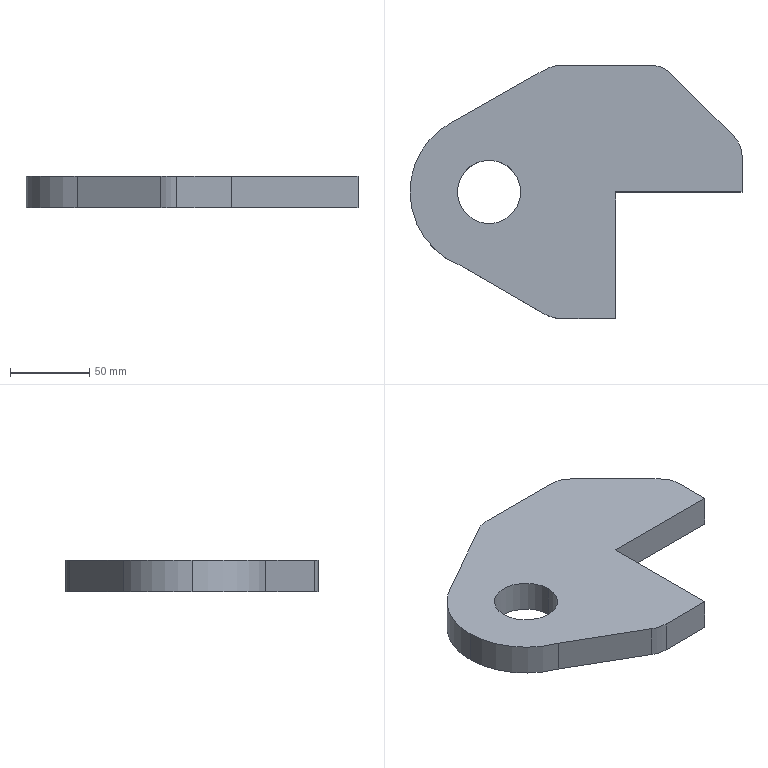Part | SolidWorks | features BaseBody 1 | 1 solid | 18 faces | box 210 x 160 x 20 mm | volume 396110 mm3 | plane 10 | cylinder 8 | commonest cylinder face diameters 40 x4 34.445 x2 100 x2
STEP:
#1=CARTESIAN_POINT('',(-20.,0.,10.));
#2=VERTEX_POINT('',#1);
#3=CARTESIAN_POINT('',(20.,0.,10.));
#4=VERTEX_POINT('',#3);
#5=CARTESIAN_POINT('',(0.,0.,10.));
#6=DIRECTION('',(0.,0.,1.));
#7=DIRECTION('',(1.,0.,0.));
#8=AXIS2_PLACEMENT_3D('',#5,#6,#7);
#9=CIRCLE('',#8,20.);
#10=EDGE_CURVE('',#2,#4,#9,.T.);
#11=ORIENTED_EDGE('',*,*,#10,.T.);
#12=CARTESIAN_POINT('',(20.,0.,-10.));
#13=VERTEX_POINT('',#12);
#14=CARTESIAN_POINT('',(20.,0.,10.));
#15=DIRECTION('',(0.,0.,-1.));
#16=VECTOR('',#15,1000.);
#17=LINE('',#14,#16);
#18=EDGE_CURVE('',#4,#13,#17,.T.);
#19=ORIENTED_EDGE('',*,*,#18,.T.);
#20=CARTESIAN_POINT('',(-20.,0.,-10.));
#21=VERTEX_POINT('',#20);
#22=CARTESIAN_POINT('',(0.,0.,-10.));
#23=DIRECTION('',(0.,0.,1.));
#24=DIRECTION('',(1.,0.,0.));
#25=AXIS2_PLACEMENT_3D('',#22,#23,#24);
#26=CIRCLE('',#25,20.);
#27=EDGE_CURVE('',#21,#13,#26,.T.);
#28=ORIENTED_EDGE('',*,*,#27,.F.);
#29=CARTESIAN_POINT('',(-20.,0.,10.));
#30=DIRECTION('',(0.,0.,-1.));
#31=VECTOR('',#30,1000.);
#32=LINE('',#29,#31);
#33=EDGE_CURVE('',#2,#21,#32,.T.);
#34=ORIENTED_EDGE('',*,*,#33,.F.);
#35=EDGE_LOOP('',(#11,#19,#28,#34));
#36=FACE_OUTER_BOUND('',#35,.T.);
#37=CARTESIAN_POINT('',(0.,0.,10.));
#38=DIRECTION('',(0.,0.,-1.));
#39=DIRECTION('',(-1.,0.,0.));
#40=AXIS2_PLACEMENT_3D('',#37,#38,#39);
#41=CYLINDRICAL_SURFACE('',#40,20.);
#42=ADVANCED_FACE('',(#36),#41,.F.);
#43=CARTESIAN_POINT('',(-50.,0.,10.));
#44=VERTEX_POINT('',#43);
#45=CARTESIAN_POINT('',(-17.72,-46.755,10.));
#46=VERTEX_POINT('',#45);
#47=CARTESIAN_POINT('',(0.,0.,10.));
#48=DIRECTION('',(0.,0.,1.));
#49=DIRECTION('',(1.,0.,0.));
#50=AXIS2_PLACEMENT_3D('',#47,#48,#49);
#51=CIRCLE('',#50,50.);
#52=EDGE_CURVE('',#44,#46,#51,.T.);
#53=ORIENTED_EDGE('',*,*,#52,.F.);
#54=CARTESIAN_POINT('',(-50.,0.,-10.));
#55=VERTEX_POINT('',#54);
#56=CARTESIAN_POINT('',(-50.,0.,10.));
#57=DIRECTION('',(0.,0.,-1.));
#58=VECTOR('',#57,1000.);
#59=LINE('',#56,#58);
#60=EDGE_CURVE('',#44,#55,#59,.T.);
#61=ORIENTED_EDGE('',*,*,#60,.T.);
#62=CARTESIAN_POINT('',(-17.72,-46.755,-10.));
#63=VERTEX_POINT('',#62);
#64=CARTESIAN_POINT('',(0.,0.,-10.));
#65=DIRECTION('',(0.,0.,1.));
#66=DIRECTION('',(1.,0.,0.));
#67=AXIS2_PLACEMENT_3D('',#64,#65,#66);
#68=CIRCLE('',#67,50.);
#69=EDGE_CURVE('',#55,#63,#68,.T.);
#70=ORIENTED_EDGE('',*,*,#69,.T.);
#71=CARTESIAN_POINT('',(-17.72,-46.755,10.));
#72=DIRECTION('',(0.,0.,-1.));
#73=VECTOR('',#72,1000.);
#74=LINE('',#71,#73);
#75=EDGE_CURVE('',#46,#63,#74,.T.);
#76=ORIENTED_EDGE('',*,*,#75,.F.);
#77=EDGE_LOOP('',(#53,#61,#70,#76));
#78=FACE_OUTER_BOUND('',#77,.T.);
#79=CARTESIAN_POINT('',(0.,0.,10.));
#80=DIRECTION('',(0.,0.,-1.));
#81=DIRECTION('',(-1.,0.,0.));
#82=AXIS2_PLACEMENT_3D('',#79,#80,#81);
#83=CYLINDRICAL_SURFACE('',#82,50.);
#84=ADVANCED_FACE('',(#78),#83,.T.);
#85=CARTESIAN_POINT('',(80.,0.,10.));
#86=VERTEX_POINT('',#85);
#87=CARTESIAN_POINT('',(80.,0.,-10.));
#88=VERTEX_POINT('',#87);
#89=CARTESIAN_POINT('',(80.,0.,10.));
#90=DIRECTION('',(0.,0.,-1.));
#91=VECTOR('',#90,1000.);
#92=LINE('',#89,#91);
#93=EDGE_CURVE('',#86,#88,#92,.T.);
#94=ORIENTED_EDGE('',*,*,#93,.F.);
#95=CARTESIAN_POINT('',(80.,-80.,10.));
#96=VERTEX_POINT('',#95);
#97=CARTESIAN_POINT('',(80.,80.,10.));
#98=DIRECTION('',(0.,1.,0.));
#99=VECTOR('',#98,1000.);
#100=LINE('',#97,#99);
#101=EDGE_CURVE('',#96,#86,#100,.T.);
#102=ORIENTED_EDGE('',*,*,#101,.F.);
#103=CARTESIAN_POINT('',(80.,-80.,-10.));
#104=VERTEX_POINT('',#103);
#105=CARTESIAN_POINT('',(80.,-80.,10.));
#106=DIRECTION('',(0.,0.,-1.));
#107=VECTOR('',#106,1000.);
#108=LINE('',#105,#107);
#109=EDGE_CURVE('',#96,#104,#108,.T.);
#110=ORIENTED_EDGE('',*,*,#109,.T.);
#111=CARTESIAN_POINT('',(80.,80.,-10.));
#112=DIRECTION('',(0.,1.,0.));
#113=VECTOR('',#112,1000.);
#114=LINE('',#111,#113);
#115=EDGE_CURVE('',#104,#88,#114,.T.);
#116=ORIENTED_EDGE('',*,*,#115,.T.);
#117=EDGE_LOOP('',(#94,#102,#110,#116));
#118=FACE_OUTER_BOUND('',#117,.T.);
#119=CARTESIAN_POINT('',(80.,80.,10.));
#120=DIRECTION('',(-1.,0.,0.));
#121=DIRECTION('',(0.,-1.,0.));
#122=AXIS2_PLACEMENT_3D('',#119,#120,#121);
#123=PLANE('',#122);
#124=ADVANCED_FACE('',(#118),#123,.F.);
#125=CARTESIAN_POINT('',(45.256,80.,10.));
#126=VERTEX_POINT('',#125);
#127=CARTESIAN_POINT('',(35.423,77.416,10.));
#128=VERTEX_POINT('',#127);
#129=CARTESIAN_POINT('',(45.256,60.,10.));
#130=DIRECTION('',(0.,0.,1.));
#131=DIRECTION('',(1.,0.,0.));
#132=AXIS2_PLACEMENT_3D('',#129,#130,#131);
#133=CIRCLE('',#132,20.);
#134=EDGE_CURVE('',#126,#128,#133,.T.);
#135=ORIENTED_EDGE('',*,*,#134,.T.);
#136=CARTESIAN_POINT('',(-24.581,43.54,10.));
#137=VERTEX_POINT('',#136);
#138=CARTESIAN_POINT('',(35.423,77.416,10.));
#139=DIRECTION('',(-0.8708,-0.4916,0.));
#140=VECTOR('',#139,1000.);
#141=LINE('',#138,#140);
#142=EDGE_CURVE('',#128,#137,#141,.T.);
#143=ORIENTED_EDGE('',*,*,#142,.T.);
#144=CARTESIAN_POINT('',(0.,0.,10.));
#145=DIRECTION('',(0.,0.,1.));
#146=DIRECTION('',(1.,0.,0.));
#147=AXIS2_PLACEMENT_3D('',#144,#145,#146);
#148=CIRCLE('',#147,50.);
#149=EDGE_CURVE('',#137,#44,#148,.T.);
#150=ORIENTED_EDGE('',*,*,#149,.T.);
#151=ORIENTED_EDGE('',*,*,#52,.T.);
#152=CARTESIAN_POINT('',(35.366,-77.331,10.));
#153=VERTEX_POINT('',#152);
#154=CARTESIAN_POINT('',(35.366,-77.331,10.));
#155=DIRECTION('',(0.8665,-0.4991,0.));
#156=VECTOR('',#155,1000.);
#157=LINE('',#154,#156);
#158=EDGE_CURVE('',#46,#153,#157,.T.);
#159=ORIENTED_EDGE('',*,*,#158,.T.);
#160=CARTESIAN_POINT('',(45.348,-80.,10.));
#161=VERTEX_POINT('',#160);
#162=CARTESIAN_POINT('',(45.348,-60.,10.));
#163=DIRECTION('',(0.,0.,1.));
#164=DIRECTION('',(1.,0.,0.));
#165=AXIS2_PLACEMENT_3D('',#162,#163,#164);
#166=CIRCLE('',#165,20.);
#167=EDGE_CURVE('',#153,#161,#166,.T.);
#168=ORIENTED_EDGE('',*,*,#167,.T.);
#169=CARTESIAN_POINT('',(80.,-80.,10.));
#170=DIRECTION('',(1.,0.,0.));
#171=VECTOR('',#170,1000.);
#172=LINE('',#169,#171);
#173=EDGE_CURVE('',#161,#96,#172,.T.);
#174=ORIENTED_EDGE('',*,*,#173,.T.);
#175=ORIENTED_EDGE('',*,*,#101,.T.);
#176=CARTESIAN_POINT('',(160.,0.,10.));
#177=VERTEX_POINT('',#176);
#178=CARTESIAN_POINT('',(160.,0.,10.));
#179=DIRECTION('',(1.,0.,0.));
#180=VECTOR('',#179,1000.);
#181=LINE('',#178,#180);
#182=EDGE_CURVE('',#86,#177,#181,.T.);
#183=ORIENTED_EDGE('',*,*,#182,.T.);
#184=CARTESIAN_POINT('',(160.,22.866,10.));
#185=VERTEX_POINT('',#184);
#186=CARTESIAN_POINT('',(160.,22.866,10.));
#187=DIRECTION('',(0.,1.,0.));
#188=VECTOR('',#187,1000.);
#189=LINE('',#186,#188);
#190=EDGE_CURVE('',#177,#185,#189,.T.);
#191=ORIENTED_EDGE('',*,*,#190,.T.);
#192=CARTESIAN_POINT('',(154.956,35.044,10.));
#193=VERTEX_POINT('',#192);
#194=CARTESIAN_POINT('',(142.778,22.866,10.));
#195=DIRECTION('',(0.,0.,1.));
#196=DIRECTION('',(-1.,0.,0.));
#197=AXIS2_PLACEMENT_3D('',#194,#195,#196);
#198=CIRCLE('',#197,17.222);
#199=EDGE_CURVE('',#185,#193,#198,.T.);
#200=ORIENTED_EDGE('',*,*,#199,.T.);
#201=CARTESIAN_POINT('',(115.044,74.956,10.));
#202=VERTEX_POINT('',#201);
#203=CARTESIAN_POINT('',(115.044,74.956,10.));
#204=DIRECTION('',(-0.7071,0.7071,0.));
#205=VECTOR('',#204,1000.);
#206=LINE('',#203,#205);
#207=EDGE_CURVE('',#193,#202,#206,.T.);
#208=ORIENTED_EDGE('',*,*,#207,.T.);
#209=CARTESIAN_POINT('',(102.866,80.,10.));
#210=VERTEX_POINT('',#209);
#211=CARTESIAN_POINT('',(102.866,62.778,10.));
#212=DIRECTION('',(0.,0.,1.));
#213=DIRECTION('',(-1.,0.,0.));
#214=AXIS2_PLACEMENT_3D('',#211,#212,#213);
#215=CIRCLE('',#214,17.222);
#216=EDGE_CURVE('',#202,#210,#215,.T.);
#217=ORIENTED_EDGE('',*,*,#216,.T.);
#218=CARTESIAN_POINT('',(80.,80.,10.));
#219=DIRECTION('',(-1.,0.,0.));
#220=VECTOR('',#219,1000.);
#221=LINE('',#218,#220);
#222=EDGE_CURVE('',#210,#126,#221,.T.);
#223=ORIENTED_EDGE('',*,*,#222,.T.);
#224=EDGE_LOOP('',(#135,#143,#150,#151,#159,#168,#174,#175,#183,#191,#200,#208,#217,#223));
#225=FACE_OUTER_BOUND('',#224,.T.);
#226=ORIENTED_EDGE('',*,*,#10,.F.);
#227=CARTESIAN_POINT('',(0.,0.,10.));
#228=DIRECTION('',(0.,0.,1.));
#229=DIRECTION('',(1.,0.,0.));
#230=AXIS2_PLACEMENT_3D('',#227,#228,#229);
#231=CIRCLE('',#230,20.);
#232=EDGE_CURVE('',#4,#2,#231,.T.);
#233=ORIENTED_EDGE('',*,*,#232,.F.);
#234=EDGE_LOOP('',(#226,#233));
#235=FACE_BOUND('',#234,.T.);
#236=CARTESIAN_POINT('',(45.256,60.,10.));
#237=DIRECTION('',(0.,0.,1.));
#238=DIRECTION('',(1.,0.,0.));
#239=AXIS2_PLACEMENT_3D('',#236,#237,#238);
#240=PLANE('',#239);
#241=ADVANCED_FACE('',(#225,#235),#240,.T.);
#242=CARTESIAN_POINT('',(45.256,80.,-10.));
#243=VERTEX_POINT('',#242);
#244=CARTESIAN_POINT('',(35.423,77.416,-10.));
#245=VERTEX_POINT('',#244);
#246=CARTESIAN_POINT('',(45.256,60.,-10.));
#247=DIRECTION('',(0.,0.,1.));
#248=DIRECTION('',(1.,0.,0.));
#249=AXIS2_PLACEMENT_3D('',#246,#247,#248);
#250=CIRCLE('',#249,20.);
#251=EDGE_CURVE('',#243,#245,#250,.T.);
#252=ORIENTED_EDGE('',*,*,#251,.F.);
#253=CARTESIAN_POINT('',(102.866,80.,-10.));
#254=VERTEX_POINT('',#253);
#255=CARTESIAN_POINT('',(80.,80.,-10.));
#256=DIRECTION('',(-1.,0.,0.));
#257=VECTOR('',#256,1000.);
#258=LINE('',#255,#257);
#259=EDGE_CURVE('',#254,#243,#258,.T.);
#260=ORIENTED_EDGE('',*,*,#259,.F.);
#261=CARTESIAN_POINT('',(115.044,74.956,-10.));
#262=VERTEX_POINT('',#261);
#263=CARTESIAN_POINT('',(102.866,62.778,-10.));
#264=DIRECTION('',(0.,0.,1.));
#265=DIRECTION('',(-1.,0.,0.));
#266=AXIS2_PLACEMENT_3D('',#263,#264,#265);
#267=CIRCLE('',#266,17.222);
#268=EDGE_CURVE('',#262,#254,#267,.T.);
#269=ORIENTED_EDGE('',*,*,#268,.F.);
#270=CARTESIAN_POINT('',(154.956,35.044,-10.));
#271=VERTEX_POINT('',#270);
#272=CARTESIAN_POINT('',(115.044,74.956,-10.));
#273=DIRECTION('',(-0.7071,0.7071,0.));
#274=VECTOR('',#273,1000.);
#275=LINE('',#272,#274);
#276=EDGE_CURVE('',#271,#262,#275,.T.);
#277=ORIENTED_EDGE('',*,*,#276,.F.);
#278=CARTESIAN_POINT('',(160.,22.866,-10.));
#279=VERTEX_POINT('',#278);
#280=CARTESIAN_POINT('',(142.778,22.866,-10.));
#281=DIRECTION('',(0.,0.,1.));
#282=DIRECTION('',(-1.,0.,0.));
#283=AXIS2_PLACEMENT_3D('',#280,#281,#282);
#284=CIRCLE('',#283,17.222);
#285=EDGE_CURVE('',#279,#271,#284,.T.);
#286=ORIENTED_EDGE('',*,*,#285,.F.);
#287=CARTESIAN_POINT('',(160.,0.,-10.));
#288=VERTEX_POINT('',#287);
#289=CARTESIAN_POINT('',(160.,22.866,-10.));
#290=DIRECTION('',(0.,1.,0.));
#291=VECTOR('',#290,1000.);
#292=LINE('',#289,#291);
#293=EDGE_CURVE('',#288,#279,#292,.T.);
#294=ORIENTED_EDGE('',*,*,#293,.F.);
#295=CARTESIAN_POINT('',(160.,0.,-10.));
#296=DIRECTION('',(1.,0.,0.));
#297=VECTOR('',#296,1000.);
#298=LINE('',#295,#297);
#299=EDGE_CURVE('',#88,#288,#298,.T.);
#300=ORIENTED_EDGE('',*,*,#299,.F.);
#301=ORIENTED_EDGE('',*,*,#115,.F.);
#302=CARTESIAN_POINT('',(45.348,-80.,-10.));
#303=VERTEX_POINT('',#302);
#304=CARTESIAN_POINT('',(80.,-80.,-10.));
#305=DIRECTION('',(1.,0.,0.));
#306=VECTOR('',#305,1000.);
#307=LINE('',#304,#306);
#308=EDGE_CURVE('',#303,#104,#307,.T.);
#309=ORIENTED_EDGE('',*,*,#308,.F.);
#310=CARTESIAN_POINT('',(35.366,-77.331,-10.));
#311=VERTEX_POINT('',#310);
#312=CARTESIAN_POINT('',(45.348,-60.,-10.));
#313=DIRECTION('',(0.,0.,1.));
#314=DIRECTION('',(1.,0.,0.));
#315=AXIS2_PLACEMENT_3D('',#312,#313,#314);
#316=CIRCLE('',#315,20.);
#317=EDGE_CURVE('',#311,#303,#316,.T.);
#318=ORIENTED_EDGE('',*,*,#317,.F.);
#319=CARTESIAN_POINT('',(35.366,-77.331,-10.));
#320=DIRECTION('',(0.8665,-0.4991,0.));
#321=VECTOR('',#320,1000.);
#322=LINE('',#319,#321);
#323=EDGE_CURVE('',#63,#311,#322,.T.);
#324=ORIENTED_EDGE('',*,*,#323,.F.);
#325=ORIENTED_EDGE('',*,*,#69,.F.);
#326=CARTESIAN_POINT('',(-24.581,43.54,-10.));
#327=VERTEX_POINT('',#326);
#328=CARTESIAN_POINT('',(0.,0.,-10.));
#329=DIRECTION('',(0.,0.,1.));
#330=DIRECTION('',(1.,0.,0.));
#331=AXIS2_PLACEMENT_3D('',#328,#329,#330);
#332=CIRCLE('',#331,50.);
#333=EDGE_CURVE('',#327,#55,#332,.T.);
#334=ORIENTED_EDGE('',*,*,#333,.F.);
#335=CARTESIAN_POINT('',(35.423,77.416,-10.));
#336=DIRECTION('',(-0.8708,-0.4916,0.));
#337=VECTOR('',#336,1000.);
#338=LINE('',#335,#337);
#339=EDGE_CURVE('',#245,#327,#338,.T.);
#340=ORIENTED_EDGE('',*,*,#339,.F.);
#341=EDGE_LOOP('',(#252,#260,#269,#277,#286,#294,#300,#301,#309,#318,#324,#325,#334,#340));
#342=FACE_OUTER_BOUND('',#341,.T.);
#343=ORIENTED_EDGE('',*,*,#27,.T.);
#344=CARTESIAN_POINT('',(0.,0.,-10.));
#345=DIRECTION('',(0.,0.,1.));
#346=DIRECTION('',(1.,0.,0.));
#347=AXIS2_PLACEMENT_3D('',#344,#345,#346);
#348=CIRCLE('',#347,20.);
#349=EDGE_CURVE('',#13,#21,#348,.T.);
#350=ORIENTED_EDGE('',*,*,#349,.T.);
#351=EDGE_LOOP('',(#343,#350));
#352=FACE_BOUND('',#351,.T.);
#353=CARTESIAN_POINT('',(45.256,60.,-10.));
#354=DIRECTION('',(0.,0.,1.));
#355=DIRECTION('',(1.,0.,0.));
#356=AXIS2_PLACEMENT_3D('',#353,#354,#355);
#357=PLANE('',#356);
#358=ADVANCED_FACE('',(#342,#352),#357,.F.);
#359=ORIENTED_EDGE('',*,*,#251,.T.);
#360=CARTESIAN_POINT('',(35.423,77.416,10.));
#361=DIRECTION('',(0.,0.,-1.));
#362=VECTOR('',#361,1000.);
#363=LINE('',#360,#362);
#364=EDGE_CURVE('',#128,#245,#363,.T.);
#365=ORIENTED_EDGE('',*,*,#364,.F.);
#366=ORIENTED_EDGE('',*,*,#134,.F.);
#367=CARTESIAN_POINT('',(45.256,80.,10.));
#368=DIRECTION('',(0.,0.,-1.));
#369=VECTOR('',#368,1000.);
#370=LINE('',#367,#369);
#371=EDGE_CURVE('',#126,#243,#370,.T.);
#372=ORIENTED_EDGE('',*,*,#371,.T.);
#373=EDGE_LOOP('',(#359,#365,#366,#372));
#374=FACE_OUTER_BOUND('',#373,.T.);
#375=CARTESIAN_POINT('',(45.256,60.,10.));
#376=DIRECTION('',(0.,0.,-1.));
#377=DIRECTION('',(-1.,0.,0.));
#378=AXIS2_PLACEMENT_3D('',#375,#376,#377);
#379=CYLINDRICAL_SURFACE('',#378,20.);
#380=ADVANCED_FACE('',(#374),#379,.T.);
#381=ORIENTED_EDGE('',*,*,#339,.T.);
#382=CARTESIAN_POINT('',(-24.581,43.54,10.));
#383=DIRECTION('',(0.,0.,-1.));
#384=VECTOR('',#383,1000.);
#385=LINE('',#382,#384);
#386=EDGE_CURVE('',#137,#327,#385,.T.);
#387=ORIENTED_EDGE('',*,*,#386,.F.);
#388=ORIENTED_EDGE('',*,*,#142,.F.);
#389=ORIENTED_EDGE('',*,*,#364,.T.);
#390=EDGE_LOOP('',(#381,#387,#388,#389));
#391=FACE_OUTER_BOUND('',#390,.T.);
#392=CARTESIAN_POINT('',(35.423,77.416,10.));
#393=DIRECTION('',(0.4916,-0.8708,0.));
#394=DIRECTION('',(0.8708,0.4916,0.));
#395=AXIS2_PLACEMENT_3D('',#392,#393,#394);
#396=PLANE('',#395);
#397=ADVANCED_FACE('',(#391),#396,.F.);
#398=ORIENTED_EDGE('',*,*,#60,.F.);
#399=ORIENTED_EDGE('',*,*,#149,.F.);
#400=ORIENTED_EDGE('',*,*,#386,.T.);
#401=ORIENTED_EDGE('',*,*,#333,.T.);
#402=EDGE_LOOP('',(#398,#399,#400,#401));
#403=FACE_OUTER_BOUND('',#402,.T.);
#404=CARTESIAN_POINT('',(0.,0.,10.));
#405=DIRECTION('',(0.,0.,-1.));
#406=DIRECTION('',(-1.,0.,0.));
#407=AXIS2_PLACEMENT_3D('',#404,#405,#406);
#408=CYLINDRICAL_SURFACE('',#407,50.);
#409=ADVANCED_FACE('',(#403),#408,.T.);
#410=ORIENTED_EDGE('',*,*,#323,.T.);
#411=CARTESIAN_POINT('',(35.366,-77.331,10.));
#412=DIRECTION('',(0.,0.,-1.));
#413=VECTOR('',#412,1000.);
#414=LINE('',#411,#413);
#415=EDGE_CURVE('',#153,#311,#414,.T.);
#416=ORIENTED_EDGE('',*,*,#415,.F.);
#417=ORIENTED_EDGE('',*,*,#158,.F.);
#418=ORIENTED_EDGE('',*,*,#75,.T.);
#419=EDGE_LOOP('',(#410,#416,#417,#418));
#420=FACE_OUTER_BOUND('',#419,.T.);
#421=CARTESIAN_POINT('',(35.366,-77.331,10.));
#422=DIRECTION('',(0.4991,0.8665,0.));
#423=DIRECTION('',(-0.8665,0.4991,0.));
#424=AXIS2_PLACEMENT_3D('',#421,#422,#423);
#425=PLANE('',#424);
#426=ADVANCED_FACE('',(#420),#425,.F.);
#427=ORIENTED_EDGE('',*,*,#317,.T.);
#428=CARTESIAN_POINT('',(45.348,-80.,10.));
#429=DIRECTION('',(0.,0.,-1.));
#430=VECTOR('',#429,1000.);
#431=LINE('',#428,#430);
#432=EDGE_CURVE('',#161,#303,#431,.T.);
#433=ORIENTED_EDGE('',*,*,#432,.F.);
#434=ORIENTED_EDGE('',*,*,#167,.F.);
#435=ORIENTED_EDGE('',*,*,#415,.T.);
#436=EDGE_LOOP('',(#427,#433,#434,#435));
#437=FACE_OUTER_BOUND('',#436,.T.);
#438=CARTESIAN_POINT('',(45.348,-60.,10.));
#439=DIRECTION('',(0.,0.,-1.));
#440=DIRECTION('',(-1.,0.,0.));
#441=AXIS2_PLACEMENT_3D('',#438,#439,#440);
#442=CYLINDRICAL_SURFACE('',#441,20.);
#443=ADVANCED_FACE('',(#437),#442,.T.);
#444=ORIENTED_EDGE('',*,*,#308,.T.);
#445=ORIENTED_EDGE('',*,*,#109,.F.);
#446=ORIENTED_EDGE('',*,*,#173,.F.);
#447=ORIENTED_EDGE('',*,*,#432,.T.);
#448=EDGE_LOOP('',(#444,#445,#446,#447));
#449=FACE_OUTER_BOUND('',#448,.T.);
#450=CARTESIAN_POINT('',(80.,-80.,10.));
#451=DIRECTION('',(0.,1.,0.));
#452=DIRECTION('',(0.,0.,1.));
#453=AXIS2_PLACEMENT_3D('',#450,#451,#452);
#454=PLANE('',#453);
#455=ADVANCED_FACE('',(#449),#454,.F.);
#456=ORIENTED_EDGE('',*,*,#259,.T.);
#457=ORIENTED_EDGE('',*,*,#371,.F.);
#458=ORIENTED_EDGE('',*,*,#222,.F.);
#459=CARTESIAN_POINT('',(102.866,80.,10.));
#460=DIRECTION('',(0.,0.,-1.));
#461=VECTOR('',#460,1000.);
#462=LINE('',#459,#461);
#463=EDGE_CURVE('',#210,#254,#462,.T.);
#464=ORIENTED_EDGE('',*,*,#463,.T.);
#465=EDGE_LOOP('',(#456,#457,#458,#464));
#466=FACE_OUTER_BOUND('',#465,.T.);
#467=CARTESIAN_POINT('',(80.,80.,10.));
#468=DIRECTION('',(0.,-1.,0.));
#469=DIRECTION('',(1.,0.,0.));
#470=AXIS2_PLACEMENT_3D('',#467,#468,#469);
#471=PLANE('',#470);
#472=ADVANCED_FACE('',(#466),#471,.F.);
#473=ORIENTED_EDGE('',*,*,#18,.F.);
#474=ORIENTED_EDGE('',*,*,#232,.T.);
#475=ORIENTED_EDGE('',*,*,#33,.T.);
#476=ORIENTED_EDGE('',*,*,#349,.F.);
#477=EDGE_LOOP('',(#473,#474,#475,#476));
#478=FACE_OUTER_BOUND('',#477,.T.);
#479=CARTESIAN_POINT('',(0.,0.,10.));
#480=DIRECTION('',(0.,0.,-1.));
#481=DIRECTION('',(-1.,0.,0.));
#482=AXIS2_PLACEMENT_3D('',#479,#480,#481);
#483=CYLINDRICAL_SURFACE('',#482,20.);
#484=ADVANCED_FACE('',(#478),#483,.F.);
#485=ORIENTED_EDGE('',*,*,#299,.T.);
#486=CARTESIAN_POINT('',(160.,0.,10.));
#487=DIRECTION('',(0.,0.,-1.));
#488=VECTOR('',#487,1000.);
#489=LINE('',#486,#488);
#490=EDGE_CURVE('',#177,#288,#489,.T.);
#491=ORIENTED_EDGE('',*,*,#490,.F.);
#492=ORIENTED_EDGE('',*,*,#182,.F.);
#493=ORIENTED_EDGE('',*,*,#93,.T.);
#494=EDGE_LOOP('',(#485,#491,#492,#493));
#495=FACE_OUTER_BOUND('',#494,.T.);
#496=CARTESIAN_POINT('',(160.,0.,10.));
#497=DIRECTION('',(0.,1.,0.));
#498=DIRECTION('',(-1.,0.,0.));
#499=AXIS2_PLACEMENT_3D('',#496,#497,#498);
#500=PLANE('',#499);
#501=ADVANCED_FACE('',(#495),#500,.F.);
#502=ORIENTED_EDGE('',*,*,#293,.T.);
#503=CARTESIAN_POINT('',(160.,22.866,10.));
#504=DIRECTION('',(0.,0.,-1.));
#505=VECTOR('',#504,1000.);
#506=LINE('',#503,#505);
#507=EDGE_CURVE('',#185,#279,#506,.T.);
#508=ORIENTED_EDGE('',*,*,#507,.F.);
#509=ORIENTED_EDGE('',*,*,#190,.F.);
#510=ORIENTED_EDGE('',*,*,#490,.T.);
#511=EDGE_LOOP('',(#502,#508,#509,#510));
#512=FACE_OUTER_BOUND('',#511,.T.);
#513=CARTESIAN_POINT('',(160.,22.866,10.));
#514=DIRECTION('',(-1.,0.,0.));
#515=DIRECTION('',(0.,0.,1.));
#516=AXIS2_PLACEMENT_3D('',#513,#514,#515);
#517=PLANE('',#516);
#518=ADVANCED_FACE('',(#512),#517,.F.);
#519=ORIENTED_EDGE('',*,*,#285,.T.);
#520=CARTESIAN_POINT('',(154.956,35.044,10.));
#521=DIRECTION('',(0.,0.,-1.));
#522=VECTOR('',#521,1000.);
#523=LINE('',#520,#522);
#524=EDGE_CURVE('',#193,#271,#523,.T.);
#525=ORIENTED_EDGE('',*,*,#524,.F.);
#526=ORIENTED_EDGE('',*,*,#199,.F.);
#527=ORIENTED_EDGE('',*,*,#507,.T.);
#528=EDGE_LOOP('',(#519,#525,#526,#527));
#529=FACE_OUTER_BOUND('',#528,.T.);
#530=CARTESIAN_POINT('',(142.778,22.866,10.));
#531=DIRECTION('',(0.,0.,-1.));
#532=DIRECTION('',(-1.,0.,0.));
#533=AXIS2_PLACEMENT_3D('',#530,#531,#532);
#534=CYLINDRICAL_SURFACE('',#533,17.222);
#535=ADVANCED_FACE('',(#529),#534,.T.);
#536=ORIENTED_EDGE('',*,*,#276,.T.);
#537=CARTESIAN_POINT('',(115.044,74.956,10.));
#538=DIRECTION('',(0.,0.,-1.));
#539=VECTOR('',#538,1000.);
#540=LINE('',#537,#539);
#541=EDGE_CURVE('',#202,#262,#540,.T.);
#542=ORIENTED_EDGE('',*,*,#541,.F.);
#543=ORIENTED_EDGE('',*,*,#207,.F.);
#544=ORIENTED_EDGE('',*,*,#524,.T.);
#545=EDGE_LOOP('',(#536,#542,#543,#544));
#546=FACE_OUTER_BOUND('',#545,.T.);
#547=CARTESIAN_POINT('',(115.044,74.956,10.));
#548=DIRECTION('',(-0.7071,-0.7071,0.));
#549=DIRECTION('',(0.7071,-0.7071,0.));
#550=AXIS2_PLACEMENT_3D('',#547,#548,#549);
#551=PLANE('',#550);
#552=ADVANCED_FACE('',(#546),#551,.F.);
#553=ORIENTED_EDGE('',*,*,#268,.T.);
#554=ORIENTED_EDGE('',*,*,#463,.F.);
#555=ORIENTED_EDGE('',*,*,#216,.F.);
#556=ORIENTED_EDGE('',*,*,#541,.T.);
#557=EDGE_LOOP('',(#553,#554,#555,#556));
#558=FACE_OUTER_BOUND('',#557,.T.);
#559=CARTESIAN_POINT('',(102.866,62.778,10.));
#560=DIRECTION('',(0.,0.,-1.));
#561=DIRECTION('',(-1.,0.,0.));
#562=AXIS2_PLACEMENT_3D('',#559,#560,#561);
#563=CYLINDRICAL_SURFACE('',#562,17.222);
#564=ADVANCED_FACE('',(#558),#563,.T.);
#565=CLOSED_SHELL('',(#42,#84,#124,#241,#358,#380,#397,#409,#426,#443,#455,#472,#484,#501,#518,#535,#552,#564));
#566=MANIFOLD_SOLID_BREP('',#565);
#567=CARTESIAN_POINT('',(0.,0.,0.));
#568=DIRECTION('',(0.,0.,1.));
#569=DIRECTION('',(1.,0.,0.));
#570=AXIS2_PLACEMENT_3D('',#567,#568,#569);
#571=(LENGTH_UNIT()NAMED_UNIT(*)SI_UNIT(.MILLI.,.METRE.));
#572=UNCERTAINTY_MEASURE_WITH_UNIT(LENGTH_MEASURE(0.00001),#571,'','');
#573=(NAMED_UNIT(*)PLANE_ANGLE_UNIT()SI_UNIT($,.RADIAN.));
#574=(NAMED_UNIT(*)SI_UNIT($,.STERADIAN.)SOLID_ANGLE_UNIT());
#575=(GEOMETRIC_REPRESENTATION_CONTEXT(3)GLOBAL_UNCERTAINTY_ASSIGNED_CONTEXT((#572))GLOBAL_UNIT_ASSIGNED_CONTEXT((#571,#573,#574))REPRESENTATION_CONTEXT('',''));
#576=ADVANCED_BREP_SHAPE_REPRESENTATION('',(#566,#570),#575);